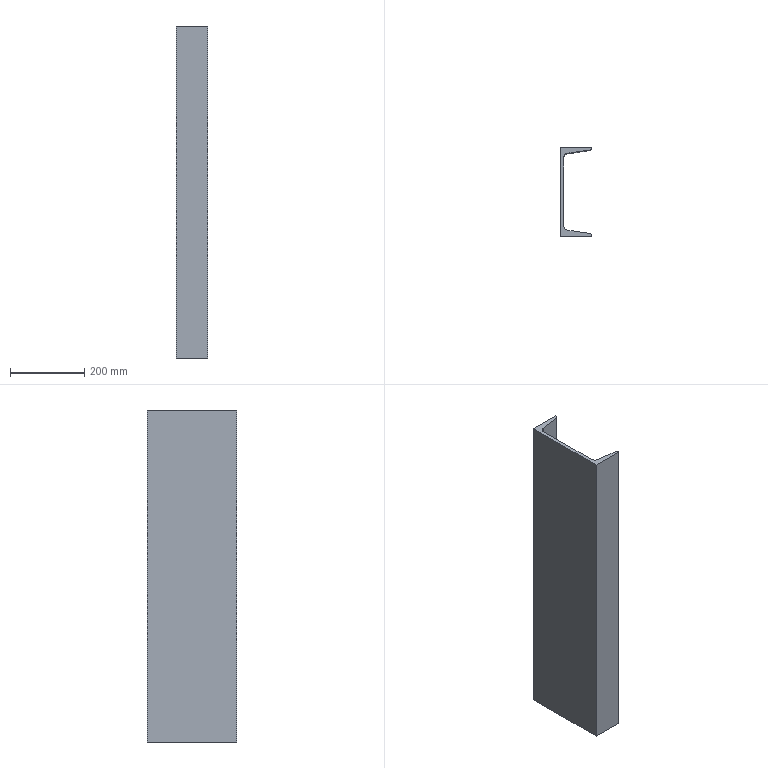Part | SolidWorks | features Extrusion 1, HoleWzd 1 | 1 solid | 22 faces | box 85 x 240 x 895 mm | volume 3741522 mm3 | plane 10 | cylinder 8 | cone 4 | commonest cylinder face diameters 5 x4 13 x2 26 x2
STEP:
#1=CARTESIAN_POINT('',(-60.,-15.,742.5));
#2=VERTEX_POINT('',#1);
#3=CARTESIAN_POINT('',(-60.,-15.,747.5));
#4=VERTEX_POINT('',#3);
#5=CARTESIAN_POINT('',(-60.,-15.,745.));
#6=DIRECTION('',(0.,1.,0.));
#7=DIRECTION('',(0.,0.,1.));
#8=AXIS2_PLACEMENT_3D('',#5,#6,#7);
#9=CIRCLE('',#8,2.5);
#10=EDGE_CURVE('',#2,#4,#9,.T.);
#11=ORIENTED_EDGE('',*,*,#10,.F.);
#12=CARTESIAN_POINT('',(-60.,0.,742.5));
#13=VERTEX_POINT('',#12);
#14=CARTESIAN_POINT('',(-60.,0.,742.5));
#15=DIRECTION('',(0.,1.,0.));
#16=VECTOR('',#15,1000.);
#17=LINE('',#14,#16);
#18=EDGE_CURVE('',#2,#13,#17,.T.);
#19=ORIENTED_EDGE('',*,*,#18,.T.);
#20=CARTESIAN_POINT('',(-60.,0.,747.5));
#21=VERTEX_POINT('',#20);
#22=CARTESIAN_POINT('',(-60.,0.,745.));
#23=DIRECTION('',(0.,1.,0.));
#24=DIRECTION('',(0.,0.,1.));
#25=AXIS2_PLACEMENT_3D('',#22,#23,#24);
#26=CIRCLE('',#25,2.5);
#27=EDGE_CURVE('',#13,#21,#26,.T.);
#28=ORIENTED_EDGE('',*,*,#27,.T.);
#29=CARTESIAN_POINT('',(-60.,0.,747.5));
#30=DIRECTION('',(0.,1.,0.));
#31=VECTOR('',#30,1000.);
#32=LINE('',#29,#31);
#33=EDGE_CURVE('',#4,#21,#32,.T.);
#34=ORIENTED_EDGE('',*,*,#33,.F.);
#35=EDGE_LOOP('',(#11,#19,#28,#34));
#36=FACE_OUTER_BOUND('',#35,.T.);
#37=CARTESIAN_POINT('',(-60.,0.,745.));
#38=DIRECTION('',(0.,1.,0.));
#39=DIRECTION('',(0.,0.,1.));
#40=AXIS2_PLACEMENT_3D('',#37,#38,#39);
#41=CYLINDRICAL_SURFACE('',#40,2.5);
#42=ADVANCED_FACE('',(#36),#41,.F.);
#43=CARTESIAN_POINT('',(-60.,-15.459,743.265));
#44=VERTEX_POINT('',#43);
#45=CARTESIAN_POINT('',(-60.,-15.459,746.735));
#46=VERTEX_POINT('',#45);
#47=CARTESIAN_POINT('',(-60.,-15.459,743.265));
#48=CARTESIAN_POINT('',(-62.365,-15.792,743.818));
#49=CARTESIAN_POINT('',(-62.365,-15.792,746.182));
#50=CARTESIAN_POINT('',(-60.,-15.459,746.735));
#51=(BOUNDED_CURVE()B_SPLINE_CURVE(3,(#47,#48,#49,#50),.UNSPECIFIED.,.F.,.F.)B_SPLINE_CURVE_WITH_KNOTS((4,4),(1.807,4.476),.UNSPECIFIED.)CURVE()GEOMETRIC_REPRESENTATION_ITEM()RATIONAL_B_SPLINE_CURVE((1.,0.4893,0.4893,1.))REPRESENTATION_ITEM(''));
#52=EDGE_CURVE('',#44,#46,#51,.T.);
#53=ORIENTED_EDGE('',*,*,#52,.F.);
#54=CARTESIAN_POINT('',(-60.,-15.,742.5));
#55=DIRECTION('',(0.,0.515,-0.8572));
#56=VECTOR('',#55,1000.);
#57=LINE('',#54,#56);
#58=EDGE_CURVE('',#44,#2,#57,.T.);
#59=ORIENTED_EDGE('',*,*,#58,.T.);
#60=ORIENTED_EDGE('',*,*,#10,.T.);
#61=CARTESIAN_POINT('',(-60.,-15.,747.5));
#62=DIRECTION('',(0.,0.515,0.8572));
#63=VECTOR('',#62,1000.);
#64=LINE('',#61,#63);
#65=EDGE_CURVE('',#46,#4,#64,.T.);
#66=ORIENTED_EDGE('',*,*,#65,.F.);
#67=EDGE_LOOP('',(#53,#59,#60,#66));
#68=FACE_OUTER_BOUND('',#67,.T.);
#69=CARTESIAN_POINT('',(-60.,-15.,745.));
#70=DIRECTION('',(0.,1.,0.));
#71=DIRECTION('',(0.,0.,1.));
#72=AXIS2_PLACEMENT_3D('',#69,#70,#71);
#73=CONICAL_SURFACE('',#72,2.5,1.03);
#74=ADVANCED_FACE('',(#68),#73,.F.);
#75=CARTESIAN_POINT('',(-60.,-15.,92.5));
#76=VERTEX_POINT('',#75);
#77=CARTESIAN_POINT('',(-60.,-15.,97.5));
#78=VERTEX_POINT('',#77);
#79=CARTESIAN_POINT('',(-60.,-15.,95.));
#80=DIRECTION('',(0.,1.,0.));
#81=DIRECTION('',(0.,0.,1.));
#82=AXIS2_PLACEMENT_3D('',#79,#80,#81);
#83=CIRCLE('',#82,2.5);
#84=EDGE_CURVE('',#76,#78,#83,.T.);
#85=ORIENTED_EDGE('',*,*,#84,.F.);
#86=CARTESIAN_POINT('',(-60.,0.,92.5));
#87=VERTEX_POINT('',#86);
#88=CARTESIAN_POINT('',(-60.,0.,92.5));
#89=DIRECTION('',(0.,1.,0.));
#90=VECTOR('',#89,1000.);
#91=LINE('',#88,#90);
#92=EDGE_CURVE('',#76,#87,#91,.T.);
#93=ORIENTED_EDGE('',*,*,#92,.T.);
#94=CARTESIAN_POINT('',(-60.,0.,97.5));
#95=VERTEX_POINT('',#94);
#96=CARTESIAN_POINT('',(-60.,0.,95.));
#97=DIRECTION('',(0.,1.,0.));
#98=DIRECTION('',(0.,0.,1.));
#99=AXIS2_PLACEMENT_3D('',#96,#97,#98);
#100=CIRCLE('',#99,2.5);
#101=EDGE_CURVE('',#87,#95,#100,.T.);
#102=ORIENTED_EDGE('',*,*,#101,.T.);
#103=CARTESIAN_POINT('',(-60.,0.,97.5));
#104=DIRECTION('',(0.,1.,0.));
#105=VECTOR('',#104,1000.);
#106=LINE('',#103,#105);
#107=EDGE_CURVE('',#78,#95,#106,.T.);
#108=ORIENTED_EDGE('',*,*,#107,.F.);
#109=EDGE_LOOP('',(#85,#93,#102,#108));
#110=FACE_OUTER_BOUND('',#109,.T.);
#111=CARTESIAN_POINT('',(-60.,0.,95.));
#112=DIRECTION('',(0.,1.,0.));
#113=DIRECTION('',(0.,0.,1.));
#114=AXIS2_PLACEMENT_3D('',#111,#112,#113);
#115=CYLINDRICAL_SURFACE('',#114,2.5);
#116=ADVANCED_FACE('',(#110),#115,.F.);
#117=CARTESIAN_POINT('',(-60.,-15.459,93.265));
#118=VERTEX_POINT('',#117);
#119=CARTESIAN_POINT('',(-60.,-15.459,96.735));
#120=VERTEX_POINT('',#119);
#121=CARTESIAN_POINT('',(-60.,-15.459,93.265));
#122=CARTESIAN_POINT('',(-62.365,-15.792,93.818));
#123=CARTESIAN_POINT('',(-62.365,-15.792,96.182));
#124=CARTESIAN_POINT('',(-60.,-15.459,96.735));
#125=(BOUNDED_CURVE()B_SPLINE_CURVE(3,(#121,#122,#123,#124),.UNSPECIFIED.,.F.,.F.)B_SPLINE_CURVE_WITH_KNOTS((4,4),(1.807,4.476),.UNSPECIFIED.)CURVE()GEOMETRIC_REPRESENTATION_ITEM()RATIONAL_B_SPLINE_CURVE((1.,0.4893,0.4893,1.))REPRESENTATION_ITEM(''));
#126=EDGE_CURVE('',#118,#120,#125,.T.);
#127=ORIENTED_EDGE('',*,*,#126,.F.);
#128=CARTESIAN_POINT('',(-60.,-15.,92.5));
#129=DIRECTION('',(0.,0.515,-0.8572));
#130=VECTOR('',#129,1000.);
#131=LINE('',#128,#130);
#132=EDGE_CURVE('',#118,#76,#131,.T.);
#133=ORIENTED_EDGE('',*,*,#132,.T.);
#134=ORIENTED_EDGE('',*,*,#84,.T.);
#135=CARTESIAN_POINT('',(-60.,-15.,97.5));
#136=DIRECTION('',(0.,0.515,0.8572));
#137=VECTOR('',#136,1000.);
#138=LINE('',#135,#137);
#139=EDGE_CURVE('',#120,#78,#138,.T.);
#140=ORIENTED_EDGE('',*,*,#139,.F.);
#141=EDGE_LOOP('',(#127,#133,#134,#140));
#142=FACE_OUTER_BOUND('',#141,.T.);
#143=CARTESIAN_POINT('',(-60.,-15.,95.));
#144=DIRECTION('',(0.,1.,0.));
#145=DIRECTION('',(0.,0.,1.));
#146=AXIS2_PLACEMENT_3D('',#143,#144,#145);
#147=CONICAL_SURFACE('',#146,2.5,1.03);
#148=ADVANCED_FACE('',(#142),#147,.F.);
#149=CARTESIAN_POINT('',(0.,-1.377,0.));
#150=VERTEX_POINT('',#149);
#151=CARTESIAN_POINT('',(0.,0.,0.));
#152=VERTEX_POINT('',#151);
#153=CARTESIAN_POINT('',(0.,-1.377,0.));
#154=DIRECTION('',(0.,1.,0.));
#155=VECTOR('',#154,1000.);
#156=LINE('',#153,#155);
#157=EDGE_CURVE('',#150,#152,#156,.T.);
#158=ORIENTED_EDGE('',*,*,#157,.T.);
#159=CARTESIAN_POINT('',(0.,0.,895.));
#160=VERTEX_POINT('',#159);
#161=CARTESIAN_POINT('',(0.,0.,895.));
#162=DIRECTION('',(0.,0.,-1.));
#163=VECTOR('',#162,1000.);
#164=LINE('',#161,#163);
#165=EDGE_CURVE('',#160,#152,#164,.T.);
#166=ORIENTED_EDGE('',*,*,#165,.F.);
#167=CARTESIAN_POINT('',(0.,-1.377,895.));
#168=VERTEX_POINT('',#167);
#169=CARTESIAN_POINT('',(0.,-1.377,895.));
#170=DIRECTION('',(0.,1.,0.));
#171=VECTOR('',#170,1000.);
#172=LINE('',#169,#171);
#173=EDGE_CURVE('',#168,#160,#172,.T.);
#174=ORIENTED_EDGE('',*,*,#173,.F.);
#175=CARTESIAN_POINT('',(0.,-1.377,895.));
#176=DIRECTION('',(0.,0.,-1.));
#177=VECTOR('',#176,1000.);
#178=LINE('',#175,#177);
#179=EDGE_CURVE('',#168,#150,#178,.T.);
#180=ORIENTED_EDGE('',*,*,#179,.T.);
#181=EDGE_LOOP('',(#158,#166,#174,#180));
#182=FACE_OUTER_BOUND('',#181,.T.);
#183=CARTESIAN_POINT('',(0.,-1.377,895.));
#184=DIRECTION('',(-1.,0.,0.));
#185=DIRECTION('',(0.,0.,1.));
#186=AXIS2_PLACEMENT_3D('',#183,#184,#185);
#187=PLANE('',#186);
#188=ADVANCED_FACE('',(#182),#187,.F.);
#189=CARTESIAN_POINT('',(-60.,0.,745.));
#190=DIRECTION('',(0.,1.,0.));
#191=DIRECTION('',(0.,0.,1.));
#192=AXIS2_PLACEMENT_3D('',#189,#190,#191);
#193=CIRCLE('',#192,2.5);
#194=EDGE_CURVE('',#21,#13,#193,.T.);
#195=ORIENTED_EDGE('',*,*,#194,.F.);
#196=ORIENTED_EDGE('',*,*,#27,.F.);
#197=EDGE_LOOP('',(#195,#196));
#198=FACE_BOUND('',#197,.T.);
#199=CARTESIAN_POINT('',(-60.,0.,95.));
#200=DIRECTION('',(0.,1.,0.));
#201=DIRECTION('',(0.,0.,1.));
#202=AXIS2_PLACEMENT_3D('',#199,#200,#201);
#203=CIRCLE('',#202,2.5);
#204=EDGE_CURVE('',#95,#87,#203,.T.);
#205=ORIENTED_EDGE('',*,*,#204,.F.);
#206=ORIENTED_EDGE('',*,*,#101,.F.);
#207=EDGE_LOOP('',(#205,#206));
#208=FACE_BOUND('',#207,.T.);
#209=CARTESIAN_POINT('',(-85.,0.,0.));
#210=VERTEX_POINT('',#209);
#211=CARTESIAN_POINT('',(0.,0.,0.));
#212=DIRECTION('',(-1.,0.,0.));
#213=VECTOR('',#212,1000.);
#214=LINE('',#211,#213);
#215=EDGE_CURVE('',#152,#210,#214,.T.);
#216=ORIENTED_EDGE('',*,*,#215,.T.);
#217=CARTESIAN_POINT('',(-85.,0.,895.));
#218=VERTEX_POINT('',#217);
#219=CARTESIAN_POINT('',(-85.,0.,895.));
#220=DIRECTION('',(0.,0.,-1.));
#221=VECTOR('',#220,1000.);
#222=LINE('',#219,#221);
#223=EDGE_CURVE('',#218,#210,#222,.T.);
#224=ORIENTED_EDGE('',*,*,#223,.F.);
#225=CARTESIAN_POINT('',(0.,0.,895.));
#226=DIRECTION('',(-1.,0.,0.));
#227=VECTOR('',#226,1000.);
#228=LINE('',#225,#227);
#229=EDGE_CURVE('',#160,#218,#228,.T.);
#230=ORIENTED_EDGE('',*,*,#229,.F.);
#231=ORIENTED_EDGE('',*,*,#165,.T.);
#232=EDGE_LOOP('',(#216,#224,#230,#231));
#233=FACE_OUTER_BOUND('',#232,.T.);
#234=CARTESIAN_POINT('',(0.,0.,895.));
#235=DIRECTION('',(0.,-1.,0.));
#236=DIRECTION('',(1.,0.,0.));
#237=AXIS2_PLACEMENT_3D('',#234,#235,#236);
#238=PLANE('',#237);
#239=ADVANCED_FACE('',(#198,#208,#233),#238,.F.);
#240=CARTESIAN_POINT('',(-85.,-240.,0.));
#241=VERTEX_POINT('',#240);
#242=CARTESIAN_POINT('',(-85.,0.,0.));
#243=DIRECTION('',(0.,-1.,0.));
#244=VECTOR('',#243,1000.);
#245=LINE('',#242,#244);
#246=EDGE_CURVE('',#210,#241,#245,.T.);
#247=ORIENTED_EDGE('',*,*,#246,.T.);
#248=CARTESIAN_POINT('',(-85.,-240.,895.));
#249=VERTEX_POINT('',#248);
#250=CARTESIAN_POINT('',(-85.,-240.,895.));
#251=DIRECTION('',(0.,0.,-1.));
#252=VECTOR('',#251,1000.);
#253=LINE('',#250,#252);
#254=EDGE_CURVE('',#249,#241,#253,.T.);
#255=ORIENTED_EDGE('',*,*,#254,.F.);
#256=CARTESIAN_POINT('',(-85.,0.,895.));
#257=DIRECTION('',(0.,-1.,0.));
#258=VECTOR('',#257,1000.);
#259=LINE('',#256,#258);
#260=EDGE_CURVE('',#218,#249,#259,.T.);
#261=ORIENTED_EDGE('',*,*,#260,.F.);
#262=ORIENTED_EDGE('',*,*,#223,.T.);
#263=EDGE_LOOP('',(#247,#255,#261,#262));
#264=FACE_OUTER_BOUND('',#263,.T.);
#265=CARTESIAN_POINT('',(-85.,0.,895.));
#266=DIRECTION('',(1.,0.,0.));
#267=DIRECTION('',(0.,1.,0.));
#268=AXIS2_PLACEMENT_3D('',#265,#266,#267);
#269=PLANE('',#268);
#270=ADVANCED_FACE('',(#264),#269,.F.);
#271=CARTESIAN_POINT('',(0.,-240.,0.));
#272=VERTEX_POINT('',#271);
#273=CARTESIAN_POINT('',(-85.,-240.,0.));
#274=DIRECTION('',(1.,0.,0.));
#275=VECTOR('',#274,1000.);
#276=LINE('',#273,#275);
#277=EDGE_CURVE('',#241,#272,#276,.T.);
#278=ORIENTED_EDGE('',*,*,#277,.T.);
#279=CARTESIAN_POINT('',(0.,-240.,895.));
#280=VERTEX_POINT('',#279);
#281=CARTESIAN_POINT('',(0.,-240.,895.));
#282=DIRECTION('',(0.,0.,-1.));
#283=VECTOR('',#282,1000.);
#284=LINE('',#281,#283);
#285=EDGE_CURVE('',#280,#272,#284,.T.);
#286=ORIENTED_EDGE('',*,*,#285,.F.);
#287=CARTESIAN_POINT('',(-85.,-240.,895.));
#288=DIRECTION('',(1.,0.,0.));
#289=VECTOR('',#288,1000.);
#290=LINE('',#287,#289);
#291=EDGE_CURVE('',#249,#280,#290,.T.);
#292=ORIENTED_EDGE('',*,*,#291,.F.);
#293=ORIENTED_EDGE('',*,*,#254,.T.);
#294=EDGE_LOOP('',(#278,#286,#292,#293));
#295=FACE_OUTER_BOUND('',#294,.T.);
#296=CARTESIAN_POINT('',(-85.,-240.,895.));
#297=DIRECTION('',(0.,1.,0.));
#298=DIRECTION('',(0.,0.,1.));
#299=AXIS2_PLACEMENT_3D('',#296,#297,#298);
#300=PLANE('',#299);
#301=ADVANCED_FACE('',(#295),#300,.F.);
#302=CARTESIAN_POINT('',(0.,-238.623,0.));
#303=VERTEX_POINT('',#302);
#304=CARTESIAN_POINT('',(0.,-240.,0.));
#305=DIRECTION('',(0.,1.,0.));
#306=VECTOR('',#305,1000.);
#307=LINE('',#304,#306);
#308=EDGE_CURVE('',#272,#303,#307,.T.);
#309=ORIENTED_EDGE('',*,*,#308,.T.);
#310=CARTESIAN_POINT('',(0.,-238.623,895.));
#311=VERTEX_POINT('',#310);
#312=CARTESIAN_POINT('',(0.,-238.623,895.));
#313=DIRECTION('',(0.,0.,-1.));
#314=VECTOR('',#313,1000.);
#315=LINE('',#312,#314);
#316=EDGE_CURVE('',#311,#303,#315,.T.);
#317=ORIENTED_EDGE('',*,*,#316,.F.);
#318=CARTESIAN_POINT('',(0.,-240.,895.));
#319=DIRECTION('',(0.,1.,0.));
#320=VECTOR('',#319,1000.);
#321=LINE('',#318,#320);
#322=EDGE_CURVE('',#280,#311,#321,.T.);
#323=ORIENTED_EDGE('',*,*,#322,.F.);
#324=ORIENTED_EDGE('',*,*,#285,.T.);
#325=EDGE_LOOP('',(#309,#317,#323,#324));
#326=FACE_OUTER_BOUND('',#325,.T.);
#327=CARTESIAN_POINT('',(0.,-240.,895.));
#328=DIRECTION('',(-1.,0.,0.));
#329=DIRECTION('',(0.,-1.,0.));
#330=AXIS2_PLACEMENT_3D('',#327,#328,#329);
#331=PLANE('',#330);
#332=ADVANCED_FACE('',(#326),#331,.F.);
#333=CARTESIAN_POINT('',(-5.595,-232.187,0.));
#334=VERTEX_POINT('',#333);
#335=CARTESIAN_POINT('',(-6.5,-238.623,0.));
#336=DIRECTION('',(0.,0.,1.));
#337=DIRECTION('',(1.,0.,0.));
#338=AXIS2_PLACEMENT_3D('',#335,#336,#337);
#339=CIRCLE('',#338,6.5);
#340=EDGE_CURVE('',#303,#334,#339,.T.);
#341=ORIENTED_EDGE('',*,*,#340,.T.);
#342=CARTESIAN_POINT('',(-5.595,-232.187,895.));
#343=VERTEX_POINT('',#342);
#344=CARTESIAN_POINT('',(-5.595,-232.187,895.));
#345=DIRECTION('',(0.,0.,-1.));
#346=VECTOR('',#345,1000.);
#347=LINE('',#344,#346);
#348=EDGE_CURVE('',#343,#334,#347,.T.);
#349=ORIENTED_EDGE('',*,*,#348,.F.);
#350=CARTESIAN_POINT('',(-6.5,-238.623,895.));
#351=DIRECTION('',(0.,0.,1.));
#352=DIRECTION('',(1.,0.,0.));
#353=AXIS2_PLACEMENT_3D('',#350,#351,#352);
#354=CIRCLE('',#353,6.5);
#355=EDGE_CURVE('',#311,#343,#354,.T.);
#356=ORIENTED_EDGE('',*,*,#355,.F.);
#357=ORIENTED_EDGE('',*,*,#316,.T.);
#358=EDGE_LOOP('',(#341,#349,#356,#357));
#359=FACE_OUTER_BOUND('',#358,.T.);
#360=CARTESIAN_POINT('',(-6.5,-238.623,895.));
#361=DIRECTION('',(0.,0.,-1.));
#362=DIRECTION('',(-1.,0.,0.));
#363=AXIS2_PLACEMENT_3D('',#360,#361,#362);
#364=CYLINDRICAL_SURFACE('',#363,6.5);
#365=ADVANCED_FACE('',(#359),#364,.T.);
#366=CARTESIAN_POINT('',(-64.309,-223.935,0.));
#367=VERTEX_POINT('',#366);
#368=CARTESIAN_POINT('',(-5.595,-232.187,0.));
#369=DIRECTION('',(-0.9903,0.1392,0.));
#370=VECTOR('',#369,1000.);
#371=LINE('',#368,#370);
#372=EDGE_CURVE('',#334,#367,#371,.T.);
#373=ORIENTED_EDGE('',*,*,#372,.T.);
#374=CARTESIAN_POINT('',(-64.309,-223.935,895.));
#375=VERTEX_POINT('',#374);
#376=CARTESIAN_POINT('',(-64.309,-223.935,895.));
#377=DIRECTION('',(0.,0.,-1.));
#378=VECTOR('',#377,1000.);
#379=LINE('',#376,#378);
#380=EDGE_CURVE('',#375,#367,#379,.T.);
#381=ORIENTED_EDGE('',*,*,#380,.F.);
#382=CARTESIAN_POINT('',(-5.595,-232.187,895.));
#383=DIRECTION('',(-0.9903,0.1392,0.));
#384=VECTOR('',#383,1000.);
#385=LINE('',#382,#384);
#386=EDGE_CURVE('',#343,#375,#385,.T.);
#387=ORIENTED_EDGE('',*,*,#386,.F.);
#388=ORIENTED_EDGE('',*,*,#348,.T.);
#389=EDGE_LOOP('',(#373,#381,#387,#388));
#390=FACE_OUTER_BOUND('',#389,.T.);
#391=CARTESIAN_POINT('',(-5.595,-232.187,895.));
#392=DIRECTION('',(-0.1392,-0.9903,0.));
#393=DIRECTION('',(0.9903,-0.1392,0.));
#394=AXIS2_PLACEMENT_3D('',#391,#392,#393);
#395=PLANE('',#394);
#396=ADVANCED_FACE('',(#390),#395,.F.);
#397=CARTESIAN_POINT('',(-75.5,-211.061,0.));
#398=VERTEX_POINT('',#397);
#399=CARTESIAN_POINT('',(-62.5,-211.061,0.));
#400=DIRECTION('',(0.,0.,-1.));
#401=DIRECTION('',(-1.,0.,0.));
#402=AXIS2_PLACEMENT_3D('',#399,#400,#401);
#403=CIRCLE('',#402,13.);
#404=EDGE_CURVE('',#367,#398,#403,.T.);
#405=ORIENTED_EDGE('',*,*,#404,.T.);
#406=CARTESIAN_POINT('',(-75.5,-211.061,895.));
#407=VERTEX_POINT('',#406);
#408=CARTESIAN_POINT('',(-75.5,-211.061,895.));
#409=DIRECTION('',(0.,0.,-1.));
#410=VECTOR('',#409,1000.);
#411=LINE('',#408,#410);
#412=EDGE_CURVE('',#407,#398,#411,.T.);
#413=ORIENTED_EDGE('',*,*,#412,.F.);
#414=CARTESIAN_POINT('',(-62.5,-211.061,895.));
#415=DIRECTION('',(0.,0.,-1.));
#416=DIRECTION('',(-1.,0.,0.));
#417=AXIS2_PLACEMENT_3D('',#414,#415,#416);
#418=CIRCLE('',#417,13.);
#419=EDGE_CURVE('',#375,#407,#418,.T.);
#420=ORIENTED_EDGE('',*,*,#419,.F.);
#421=ORIENTED_EDGE('',*,*,#380,.T.);
#422=EDGE_LOOP('',(#405,#413,#420,#421));
#423=FACE_OUTER_BOUND('',#422,.T.);
#424=CARTESIAN_POINT('',(-62.5,-211.061,895.));
#425=DIRECTION('',(0.,0.,-1.));
#426=DIRECTION('',(-1.,0.,0.));
#427=AXIS2_PLACEMENT_3D('',#424,#425,#426);
#428=CYLINDRICAL_SURFACE('',#427,13.);
#429=ADVANCED_FACE('',(#423),#428,.F.);
#430=CARTESIAN_POINT('',(-75.5,-28.939,0.));
#431=VERTEX_POINT('',#430);
#432=CARTESIAN_POINT('',(-75.5,-211.061,0.));
#433=DIRECTION('',(0.,1.,0.));
#434=VECTOR('',#433,1000.);
#435=LINE('',#432,#434);
#436=EDGE_CURVE('',#398,#431,#435,.T.);
#437=ORIENTED_EDGE('',*,*,#436,.T.);
#438=CARTESIAN_POINT('',(-75.5,-28.939,895.));
#439=VERTEX_POINT('',#438);
#440=CARTESIAN_POINT('',(-75.5,-28.939,895.));
#441=DIRECTION('',(0.,0.,-1.));
#442=VECTOR('',#441,1000.);
#443=LINE('',#440,#442);
#444=EDGE_CURVE('',#439,#431,#443,.T.);
#445=ORIENTED_EDGE('',*,*,#444,.F.);
#446=CARTESIAN_POINT('',(-75.5,-211.061,895.));
#447=DIRECTION('',(0.,1.,0.));
#448=VECTOR('',#447,1000.);
#449=LINE('',#446,#448);
#450=EDGE_CURVE('',#407,#439,#449,.T.);
#451=ORIENTED_EDGE('',*,*,#450,.F.);
#452=ORIENTED_EDGE('',*,*,#412,.T.);
#453=EDGE_LOOP('',(#437,#445,#451,#452));
#454=FACE_OUTER_BOUND('',#453,.T.);
#455=CARTESIAN_POINT('',(-75.5,-211.061,895.));
#456=DIRECTION('',(-1.,0.,0.));
#457=DIRECTION('',(0.,0.,1.));
#458=AXIS2_PLACEMENT_3D('',#455,#456,#457);
#459=PLANE('',#458);
#460=ADVANCED_FACE('',(#454),#459,.F.);
#461=CARTESIAN_POINT('',(-64.309,-16.065,0.));
#462=VERTEX_POINT('',#461);
#463=CARTESIAN_POINT('',(-62.5,-28.939,0.));
#464=DIRECTION('',(0.,0.,-1.));
#465=DIRECTION('',(-1.,0.,0.));
#466=AXIS2_PLACEMENT_3D('',#463,#464,#465);
#467=CIRCLE('',#466,13.);
#468=EDGE_CURVE('',#431,#462,#467,.T.);
#469=ORIENTED_EDGE('',*,*,#468,.T.);
#470=CARTESIAN_POINT('',(-64.309,-16.065,895.));
#471=VERTEX_POINT('',#470);
#472=CARTESIAN_POINT('',(-64.309,-16.065,895.));
#473=DIRECTION('',(0.,0.,-1.));
#474=VECTOR('',#473,1000.);
#475=LINE('',#472,#474);
#476=EDGE_CURVE('',#471,#462,#475,.T.);
#477=ORIENTED_EDGE('',*,*,#476,.F.);
#478=CARTESIAN_POINT('',(-62.5,-28.939,895.));
#479=DIRECTION('',(0.,0.,-1.));
#480=DIRECTION('',(-1.,0.,0.));
#481=AXIS2_PLACEMENT_3D('',#478,#479,#480);
#482=CIRCLE('',#481,13.);
#483=EDGE_CURVE('',#439,#471,#482,.T.);
#484=ORIENTED_EDGE('',*,*,#483,.F.);
#485=ORIENTED_EDGE('',*,*,#444,.T.);
#486=EDGE_LOOP('',(#469,#477,#484,#485));
#487=FACE_OUTER_BOUND('',#486,.T.);
#488=CARTESIAN_POINT('',(-62.5,-28.939,895.));
#489=DIRECTION('',(0.,0.,-1.));
#490=DIRECTION('',(-1.,0.,0.));
#491=AXIS2_PLACEMENT_3D('',#488,#489,#490);
#492=CYLINDRICAL_SURFACE('',#491,13.);
#493=ADVANCED_FACE('',(#487),#492,.F.);
#494=CARTESIAN_POINT('',(-60.,-15.459,746.735));
#495=CARTESIAN_POINT('',(-58.747,-15.283,747.028));
#496=CARTESIAN_POINT('',(-57.735,-15.141,746.253));
#497=CARTESIAN_POINT('',(-57.735,-15.141,745.));
#498=CARTESIAN_POINT('',(-57.735,-15.141,743.747));
#499=CARTESIAN_POINT('',(-58.747,-15.283,742.972));
#500=CARTESIAN_POINT('',(-60.,-15.459,743.265));
#501=(BOUNDED_CURVE()B_SPLINE_CURVE(3,(#494,#495,#496,#497,#498,#499,#500),.UNSPECIFIED.,.F.,.T.)B_SPLINE_CURVE_WITH_KNOTS((4,3,4),(4.476,6.283,8.09),.UNSPECIFIED.)CURVE()GEOMETRIC_REPRESENTATION_ITEM()RATIONAL_B_SPLINE_CURVE((1.,0.7459,0.7459,1.,0.7459,0.7459,1.))REPRESENTATION_ITEM(''));
#502=EDGE_CURVE('',#46,#44,#501,.T.);
#503=ORIENTED_EDGE('',*,*,#502,.T.);
#504=ORIENTED_EDGE('',*,*,#52,.T.);
#505=EDGE_LOOP('',(#503,#504));
#506=FACE_BOUND('',#505,.T.);
#507=CARTESIAN_POINT('',(-60.,-15.459,96.735));
#508=CARTESIAN_POINT('',(-58.747,-15.283,97.028));
#509=CARTESIAN_POINT('',(-57.735,-15.141,96.253));
#510=CARTESIAN_POINT('',(-57.735,-15.141,95.));
#511=CARTESIAN_POINT('',(-57.735,-15.141,93.747));
#512=CARTESIAN_POINT('',(-58.747,-15.283,92.972));
#513=CARTESIAN_POINT('',(-60.,-15.459,93.265));
#514=(BOUNDED_CURVE()B_SPLINE_CURVE(3,(#507,#508,#509,#510,#511,#512,#513),.UNSPECIFIED.,.F.,.F.)B_SPLINE_CURVE_WITH_KNOTS((4,3,4),(4.476,6.283,8.09),.UNSPECIFIED.)CURVE()GEOMETRIC_REPRESENTATION_ITEM()RATIONAL_B_SPLINE_CURVE((1.,0.7459,0.7459,1.,0.7459,0.7459,1.))REPRESENTATION_ITEM(''));
#515=EDGE_CURVE('',#120,#118,#514,.T.);
#516=ORIENTED_EDGE('',*,*,#515,.T.);
#517=ORIENTED_EDGE('',*,*,#126,.T.);
#518=EDGE_LOOP('',(#516,#517));
#519=FACE_BOUND('',#518,.T.);
#520=CARTESIAN_POINT('',(-5.595,-7.813,0.));
#521=VERTEX_POINT('',#520);
#522=CARTESIAN_POINT('',(-64.309,-16.065,0.));
#523=DIRECTION('',(0.9903,0.1392,0.));
#524=VECTOR('',#523,1000.);
#525=LINE('',#522,#524);
#526=EDGE_CURVE('',#462,#521,#525,.T.);
#527=ORIENTED_EDGE('',*,*,#526,.T.);
#528=CARTESIAN_POINT('',(-5.595,-7.813,895.));
#529=VERTEX_POINT('',#528);
#530=CARTESIAN_POINT('',(-5.595,-7.813,895.));
#531=DIRECTION('',(0.,0.,-1.));
#532=VECTOR('',#531,1000.);
#533=LINE('',#530,#532);
#534=EDGE_CURVE('',#529,#521,#533,.T.);
#535=ORIENTED_EDGE('',*,*,#534,.F.);
#536=CARTESIAN_POINT('',(-64.309,-16.065,895.));
#537=DIRECTION('',(0.9903,0.1392,0.));
#538=VECTOR('',#537,1000.);
#539=LINE('',#536,#538);
#540=EDGE_CURVE('',#471,#529,#539,.T.);
#541=ORIENTED_EDGE('',*,*,#540,.F.);
#542=ORIENTED_EDGE('',*,*,#476,.T.);
#543=EDGE_LOOP('',(#527,#535,#541,#542));
#544=FACE_OUTER_BOUND('',#543,.T.);
#545=CARTESIAN_POINT('',(-64.309,-16.065,895.));
#546=DIRECTION('',(-0.1392,0.9903,0.));
#547=DIRECTION('',(-0.9903,-0.1392,0.));
#548=AXIS2_PLACEMENT_3D('',#545,#546,#547);
#549=PLANE('',#548);
#550=ADVANCED_FACE('',(#506,#519,#544),#549,.F.);
#551=CARTESIAN_POINT('',(-6.5,-1.377,0.));
#552=DIRECTION('',(0.,0.,1.));
#553=DIRECTION('',(1.,0.,0.));
#554=AXIS2_PLACEMENT_3D('',#551,#552,#553);
#555=CIRCLE('',#554,6.5);
#556=EDGE_CURVE('',#521,#150,#555,.T.);
#557=ORIENTED_EDGE('',*,*,#556,.T.);
#558=ORIENTED_EDGE('',*,*,#179,.F.);
#559=CARTESIAN_POINT('',(-6.5,-1.377,895.));
#560=DIRECTION('',(0.,0.,1.));
#561=DIRECTION('',(1.,0.,0.));
#562=AXIS2_PLACEMENT_3D('',#559,#560,#561);
#563=CIRCLE('',#562,6.5);
#564=EDGE_CURVE('',#529,#168,#563,.T.);
#565=ORIENTED_EDGE('',*,*,#564,.F.);
#566=ORIENTED_EDGE('',*,*,#534,.T.);
#567=EDGE_LOOP('',(#557,#558,#565,#566));
#568=FACE_OUTER_BOUND('',#567,.T.);
#569=CARTESIAN_POINT('',(-6.5,-1.377,895.));
#570=DIRECTION('',(0.,0.,-1.));
#571=DIRECTION('',(-1.,0.,0.));
#572=AXIS2_PLACEMENT_3D('',#569,#570,#571);
#573=CYLINDRICAL_SURFACE('',#572,6.5);
#574=ADVANCED_FACE('',(#568),#573,.T.);
#575=ORIENTED_EDGE('',*,*,#173,.T.);
#576=ORIENTED_EDGE('',*,*,#229,.T.);
#577=ORIENTED_EDGE('',*,*,#260,.T.);
#578=ORIENTED_EDGE('',*,*,#291,.T.);
#579=ORIENTED_EDGE('',*,*,#322,.T.);
#580=ORIENTED_EDGE('',*,*,#355,.T.);
#581=ORIENTED_EDGE('',*,*,#386,.T.);
#582=ORIENTED_EDGE('',*,*,#419,.T.);
#583=ORIENTED_EDGE('',*,*,#450,.T.);
#584=ORIENTED_EDGE('',*,*,#483,.T.);
#585=ORIENTED_EDGE('',*,*,#540,.T.);
#586=ORIENTED_EDGE('',*,*,#564,.T.);
#587=EDGE_LOOP('',(#575,#576,#577,#578,#579,#580,#581,#582,#583,#584,#585,#586));
#588=FACE_OUTER_BOUND('',#587,.T.);
#589=CARTESIAN_POINT('',(-6.5,-238.623,895.));
#590=DIRECTION('',(0.,0.,1.));
#591=DIRECTION('',(1.,0.,0.));
#592=AXIS2_PLACEMENT_3D('',#589,#590,#591);
#593=PLANE('',#592);
#594=ADVANCED_FACE('',(#588),#593,.T.);
#595=ORIENTED_EDGE('',*,*,#157,.F.);
#596=ORIENTED_EDGE('',*,*,#556,.F.);
#597=ORIENTED_EDGE('',*,*,#526,.F.);
#598=ORIENTED_EDGE('',*,*,#468,.F.);
#599=ORIENTED_EDGE('',*,*,#436,.F.);
#600=ORIENTED_EDGE('',*,*,#404,.F.);
#601=ORIENTED_EDGE('',*,*,#372,.F.);
#602=ORIENTED_EDGE('',*,*,#340,.F.);
#603=ORIENTED_EDGE('',*,*,#308,.F.);
#604=ORIENTED_EDGE('',*,*,#277,.F.);
#605=ORIENTED_EDGE('',*,*,#246,.F.);
#606=ORIENTED_EDGE('',*,*,#215,.F.);
#607=EDGE_LOOP('',(#595,#596,#597,#598,#599,#600,#601,#602,#603,#604,#605,#606));
#608=FACE_OUTER_BOUND('',#607,.T.);
#609=CARTESIAN_POINT('',(-6.5,-238.623,0.));
#610=DIRECTION('',(0.,0.,1.));
#611=DIRECTION('',(1.,0.,0.));
#612=AXIS2_PLACEMENT_3D('',#609,#610,#611);
#613=PLANE('',#612);
#614=ADVANCED_FACE('',(#608),#613,.F.);
#615=ORIENTED_EDGE('',*,*,#132,.F.);
#616=ORIENTED_EDGE('',*,*,#515,.F.);
#617=ORIENTED_EDGE('',*,*,#139,.T.);
#618=CARTESIAN_POINT('',(-60.,-15.,95.));
#619=DIRECTION('',(0.,1.,0.));
#620=DIRECTION('',(0.,0.,1.));
#621=AXIS2_PLACEMENT_3D('',#618,#619,#620);
#622=CIRCLE('',#621,2.5);
#623=EDGE_CURVE('',#78,#76,#622,.T.);
#624=ORIENTED_EDGE('',*,*,#623,.T.);
#625=EDGE_LOOP('',(#615,#616,#617,#624));
#626=FACE_OUTER_BOUND('',#625,.T.);
#627=CARTESIAN_POINT('',(-60.,-15.,95.));
#628=DIRECTION('',(0.,1.,0.));
#629=DIRECTION('',(0.,0.,1.));
#630=AXIS2_PLACEMENT_3D('',#627,#628,#629);
#631=CONICAL_SURFACE('',#630,2.5,1.03);
#632=ADVANCED_FACE('',(#626),#631,.F.);
#633=ORIENTED_EDGE('',*,*,#92,.F.);
#634=ORIENTED_EDGE('',*,*,#623,.F.);
#635=ORIENTED_EDGE('',*,*,#107,.T.);
#636=ORIENTED_EDGE('',*,*,#204,.T.);
#637=EDGE_LOOP('',(#633,#634,#635,#636));
#638=FACE_OUTER_BOUND('',#637,.T.);
#639=CARTESIAN_POINT('',(-60.,0.,95.));
#640=DIRECTION('',(0.,1.,0.));
#641=DIRECTION('',(0.,0.,1.));
#642=AXIS2_PLACEMENT_3D('',#639,#640,#641);
#643=CYLINDRICAL_SURFACE('',#642,2.5);
#644=ADVANCED_FACE('',(#638),#643,.F.);
#645=ORIENTED_EDGE('',*,*,#58,.F.);
#646=ORIENTED_EDGE('',*,*,#502,.F.);
#647=ORIENTED_EDGE('',*,*,#65,.T.);
#648=CARTESIAN_POINT('',(-60.,-15.,745.));
#649=DIRECTION('',(0.,1.,0.));
#650=DIRECTION('',(0.,0.,1.));
#651=AXIS2_PLACEMENT_3D('',#648,#649,#650);
#652=CIRCLE('',#651,2.5);
#653=EDGE_CURVE('',#4,#2,#652,.T.);
#654=ORIENTED_EDGE('',*,*,#653,.T.);
#655=EDGE_LOOP('',(#645,#646,#647,#654));
#656=FACE_OUTER_BOUND('',#655,.T.);
#657=CARTESIAN_POINT('',(-60.,-15.,745.));
#658=DIRECTION('',(0.,1.,0.));
#659=DIRECTION('',(0.,0.,1.));
#660=AXIS2_PLACEMENT_3D('',#657,#658,#659);
#661=CONICAL_SURFACE('',#660,2.5,1.03);
#662=ADVANCED_FACE('',(#656),#661,.F.);
#663=ORIENTED_EDGE('',*,*,#18,.F.);
#664=ORIENTED_EDGE('',*,*,#653,.F.);
#665=ORIENTED_EDGE('',*,*,#33,.T.);
#666=ORIENTED_EDGE('',*,*,#194,.T.);
#667=EDGE_LOOP('',(#663,#664,#665,#666));
#668=FACE_OUTER_BOUND('',#667,.T.);
#669=CARTESIAN_POINT('',(-60.,0.,745.));
#670=DIRECTION('',(0.,1.,0.));
#671=DIRECTION('',(0.,0.,1.));
#672=AXIS2_PLACEMENT_3D('',#669,#670,#671);
#673=CYLINDRICAL_SURFACE('',#672,2.5);
#674=ADVANCED_FACE('',(#668),#673,.F.);
#675=CLOSED_SHELL('',(#42,#74,#116,#148,#188,#239,#270,#301,#332,#365,#396,#429,#460,#493,#550,#574,#594,#614,#632,#644,#662,#674));
#676=MANIFOLD_SOLID_BREP('',#675);
#677=CARTESIAN_POINT('',(0.,0.,0.));
#678=DIRECTION('',(0.,0.,1.));
#679=DIRECTION('',(1.,0.,0.));
#680=AXIS2_PLACEMENT_3D('',#677,#678,#679);
#681=(LENGTH_UNIT()NAMED_UNIT(*)SI_UNIT(.MILLI.,.METRE.));
#682=UNCERTAINTY_MEASURE_WITH_UNIT(LENGTH_MEASURE(0.00001),#681,'','');
#683=(NAMED_UNIT(*)PLANE_ANGLE_UNIT()SI_UNIT($,.RADIAN.));
#684=(NAMED_UNIT(*)SI_UNIT($,.STERADIAN.)SOLID_ANGLE_UNIT());
#685=(GEOMETRIC_REPRESENTATION_CONTEXT(3)GLOBAL_UNCERTAINTY_ASSIGNED_CONTEXT((#682))GLOBAL_UNIT_ASSIGNED_CONTEXT((#681,#683,#684))REPRESENTATION_CONTEXT('',''));
#686=ADVANCED_BREP_SHAPE_REPRESENTATION('',(#676,#680),#685);